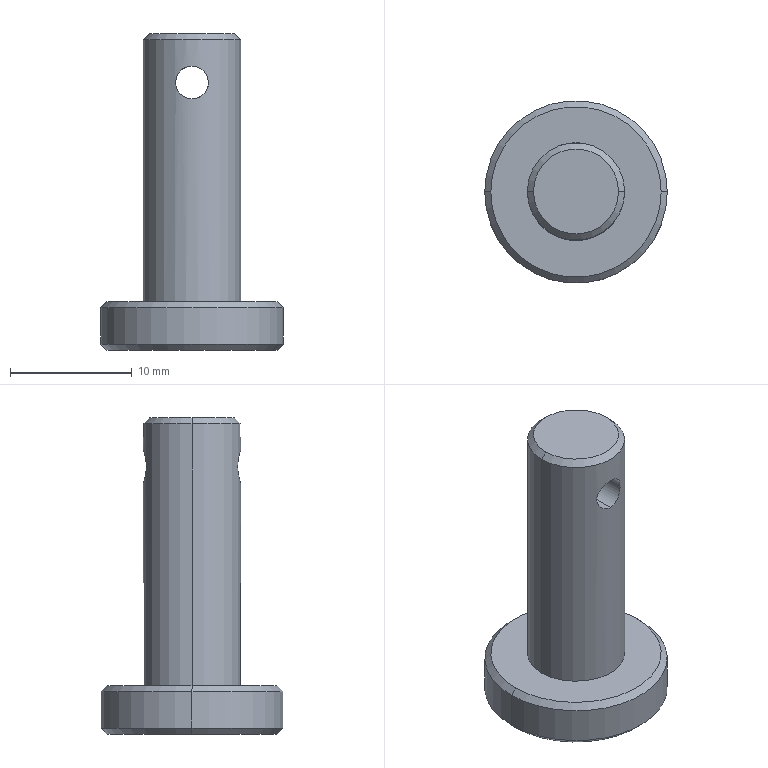Part | SolidWorks | features ICE 2, Chamfer 1, Extrusion 1 | 1 solid | 15 faces | box 15 x 15 x 26 mm | volume 1753 mm3 | cone 6 | cylinder 6 | plane 3 | commonest cylinder face diameters 2.7 x2 8 x2 15 x2
STEP:
#1=CARTESIAN_POINT('',(3.5,0.,22.));
#2=VERTEX_POINT('',#1);
#3=CARTESIAN_POINT('',(-3.5,0.,22.));
#4=VERTEX_POINT('',#3);
#5=CARTESIAN_POINT('',(0.,0.,22.));
#6=DIRECTION('',(0.,0.,1.));
#7=DIRECTION('',(1.,0.,0.));
#8=AXIS2_PLACEMENT_3D('',#5,#6,#7);
#9=CIRCLE('',#8,3.5);
#10=EDGE_CURVE('',#2,#4,#9,.T.);
#11=ORIENTED_EDGE('',*,*,#10,.F.);
#12=CARTESIAN_POINT('',(4.,0.,21.5));
#13=VERTEX_POINT('',#12);
#14=CARTESIAN_POINT('',(3.5,0.,22.));
#15=DIRECTION('',(0.7071,0.,-0.7071));
#16=VECTOR('',#15,1000.);
#17=LINE('',#14,#16);
#18=EDGE_CURVE('',#2,#13,#17,.T.);
#19=ORIENTED_EDGE('',*,*,#18,.T.);
#20=CARTESIAN_POINT('',(-4.,0.,21.5));
#21=VERTEX_POINT('',#20);
#22=CARTESIAN_POINT('',(0.,0.,21.5));
#23=DIRECTION('',(0.,0.,-1.));
#24=DIRECTION('',(1.,0.,0.));
#25=AXIS2_PLACEMENT_3D('',#22,#23,#24);
#26=CIRCLE('',#25,4.);
#27=EDGE_CURVE('',#21,#13,#26,.T.);
#28=ORIENTED_EDGE('',*,*,#27,.F.);
#29=CARTESIAN_POINT('',(-3.5,0.,22.));
#30=DIRECTION('',(-0.7071,0.,-0.7071));
#31=VECTOR('',#30,1000.);
#32=LINE('',#29,#31);
#33=EDGE_CURVE('',#4,#21,#32,.T.);
#34=ORIENTED_EDGE('',*,*,#33,.F.);
#35=EDGE_LOOP('',(#11,#19,#28,#34));
#36=FACE_OUTER_BOUND('',#35,.T.);
#37=CARTESIAN_POINT('',(0.,0.,22.));
#38=DIRECTION('',(0.,0.,-1.));
#39=DIRECTION('',(-1.,0.,0.));
#40=AXIS2_PLACEMENT_3D('',#37,#38,#39);
#41=CONICAL_SURFACE('',#40,3.5,0.7854);
#42=ADVANCED_FACE('',(#36),#41,.T.);
#43=CARTESIAN_POINT('',(7.,0.,0.));
#44=VERTEX_POINT('',#43);
#45=CARTESIAN_POINT('',(-7.,0.,0.));
#46=VERTEX_POINT('',#45);
#47=CARTESIAN_POINT('',(0.,0.,0.));
#48=DIRECTION('',(0.,0.,1.));
#49=DIRECTION('',(-1.,0.,0.));
#50=AXIS2_PLACEMENT_3D('',#47,#48,#49);
#51=CIRCLE('',#50,7.);
#52=EDGE_CURVE('',#44,#46,#51,.T.);
#53=ORIENTED_EDGE('',*,*,#52,.F.);
#54=CARTESIAN_POINT('',(7.5,0.,-0.5));
#55=VERTEX_POINT('',#54);
#56=CARTESIAN_POINT('',(7.5,0.,-0.5));
#57=DIRECTION('',(0.7071,0.,-0.7071));
#58=VECTOR('',#57,1000.);
#59=LINE('',#56,#58);
#60=EDGE_CURVE('',#44,#55,#59,.T.);
#61=ORIENTED_EDGE('',*,*,#60,.T.);
#62=CARTESIAN_POINT('',(-7.5,0.,-0.5));
#63=VERTEX_POINT('',#62);
#64=CARTESIAN_POINT('',(0.,0.,-0.5));
#65=DIRECTION('',(0.,0.,-1.));
#66=DIRECTION('',(-1.,0.,0.));
#67=AXIS2_PLACEMENT_3D('',#64,#65,#66);
#68=CIRCLE('',#67,7.5);
#69=EDGE_CURVE('',#63,#55,#68,.T.);
#70=ORIENTED_EDGE('',*,*,#69,.F.);
#71=CARTESIAN_POINT('',(-7.5,0.,-0.5));
#72=DIRECTION('',(-0.7071,0.,-0.7071));
#73=VECTOR('',#72,1000.);
#74=LINE('',#71,#73);
#75=EDGE_CURVE('',#46,#63,#74,.T.);
#76=ORIENTED_EDGE('',*,*,#75,.F.);
#77=EDGE_LOOP('',(#53,#61,#70,#76));
#78=FACE_OUTER_BOUND('',#77,.T.);
#79=CARTESIAN_POINT('',(0.,0.,-0.5));
#80=DIRECTION('',(0.,0.,-1.));
#81=DIRECTION('',(-1.,0.,0.));
#82=AXIS2_PLACEMENT_3D('',#79,#80,#81);
#83=CONICAL_SURFACE('',#82,7.5,0.7854);
#84=ADVANCED_FACE('',(#78),#83,.T.);
#85=CARTESIAN_POINT('',(-7.,0.,-4.));
#86=VERTEX_POINT('',#85);
#87=CARTESIAN_POINT('',(7.,0.,-4.));
#88=VERTEX_POINT('',#87);
#89=CARTESIAN_POINT('',(0.,0.,-4.));
#90=DIRECTION('',(0.,0.,-1.));
#91=DIRECTION('',(-1.,0.,0.));
#92=AXIS2_PLACEMENT_3D('',#89,#90,#91);
#93=CIRCLE('',#92,7.);
#94=EDGE_CURVE('',#86,#88,#93,.T.);
#95=ORIENTED_EDGE('',*,*,#94,.F.);
#96=CARTESIAN_POINT('',(-7.5,0.,-3.5));
#97=VERTEX_POINT('',#96);
#98=CARTESIAN_POINT('',(-7.,0.,-4.));
#99=DIRECTION('',(-0.7071,0.,0.7071));
#100=VECTOR('',#99,1000.);
#101=LINE('',#98,#100);
#102=EDGE_CURVE('',#86,#97,#101,.T.);
#103=ORIENTED_EDGE('',*,*,#102,.T.);
#104=CARTESIAN_POINT('',(7.5,0.,-3.5));
#105=VERTEX_POINT('',#104);
#106=CARTESIAN_POINT('',(0.,0.,-3.5));
#107=DIRECTION('',(0.,0.,1.));
#108=DIRECTION('',(-1.,0.,0.));
#109=AXIS2_PLACEMENT_3D('',#106,#107,#108);
#110=CIRCLE('',#109,7.5);
#111=EDGE_CURVE('',#105,#97,#110,.T.);
#112=ORIENTED_EDGE('',*,*,#111,.F.);
#113=CARTESIAN_POINT('',(7.,0.,-4.));
#114=DIRECTION('',(0.7071,0.,0.7071));
#115=VECTOR('',#114,1000.);
#116=LINE('',#113,#115);
#117=EDGE_CURVE('',#88,#105,#116,.T.);
#118=ORIENTED_EDGE('',*,*,#117,.F.);
#119=EDGE_LOOP('',(#95,#103,#112,#118));
#120=FACE_OUTER_BOUND('',#119,.T.);
#121=CARTESIAN_POINT('',(0.,0.,-4.));
#122=DIRECTION('',(0.,0.,1.));
#123=DIRECTION('',(1.,0.,0.));
#124=AXIS2_PLACEMENT_3D('',#121,#122,#123);
#125=CONICAL_SURFACE('',#124,7.,0.7854);
#126=ADVANCED_FACE('',(#120),#125,.T.);
#127=CARTESIAN_POINT('',(0.,-4.,16.65));
#128=VERTEX_POINT('',#127);
#129=CARTESIAN_POINT('',(0.,-4.,19.35));
#130=VERTEX_POINT('',#129);
#131=CARTESIAN_POINT('',(0.,-4.,16.65));
#132=CARTESIAN_POINT('',(-0.1771,-4.,16.65));
#133=CARTESIAN_POINT('',(-0.3558,-3.988,16.686));
#134=CARTESIAN_POINT('',(-0.6002,-3.956,16.788));
#135=CARTESIAN_POINT('',(-0.6792,-3.943,16.83));
#136=CARTESIAN_POINT('',(-0.8249,-3.915,16.928));
#137=CARTESIAN_POINT('',(-0.8925,-3.9,16.983));
#138=CARTESIAN_POINT('',(-1.079,-3.854,17.17));
#139=CARTESIAN_POINT('',(-1.178,-3.823,17.318));
#140=CARTESIAN_POINT('',(-1.281,-3.79,17.564));
#141=CARTESIAN_POINT('',(-1.306,-3.781,17.648));
#142=CARTESIAN_POINT('',(-1.341,-3.769,17.821));
#143=CARTESIAN_POINT('',(-1.35,-3.765,17.911));
#144=CARTESIAN_POINT('',(-1.35,-3.765,18.178));
#145=CARTESIAN_POINT('',(-1.314,-3.779,18.356));
#146=CARTESIAN_POINT('',(-1.179,-3.823,18.681));
#147=CARTESIAN_POINT('',(-1.078,-3.854,18.831));
#148=CARTESIAN_POINT('',(-0.8929,-3.9,19.016));
#149=CARTESIAN_POINT('',(-0.8239,-3.915,19.073));
#150=CARTESIAN_POINT('',(-0.6781,-3.943,19.171));
#151=CARTESIAN_POINT('',(-0.6009,-3.955,19.212));
#152=CARTESIAN_POINT('',(-0.4376,-3.977,19.28));
#153=CARTESIAN_POINT('',(-0.3516,-3.985,19.306));
#154=CARTESIAN_POINT('',(-0.1782,-3.997,19.341));
#155=CARTESIAN_POINT('',(-0.08989,-4.,19.35));
#156=CARTESIAN_POINT('',(0.,-4.,19.35));
#157=B_SPLINE_CURVE_WITH_KNOTS('',3,(#131,#132,#133,#134,#135,#136,#137,#138,#139,#140,#141,#142,#143,#144,#145,#146,#147,#148,#149,#150,#151,#152,#153,#154,#155,#156),.UNSPECIFIED.,.F.,.F.,(4,2,2,2,2,2,2,2,2,2,2,2,4),(0.004252,0.004784,0.005049,0.005315,0.005846,0.006112,0.006378,0.006909,0.007441,0.007706,0.007972,0.008238,0.008503),.UNSPECIFIED.);
#158=EDGE_CURVE('',#128,#130,#157,.T.);
#159=ORIENTED_EDGE('',*,*,#158,.F.);
#160=CARTESIAN_POINT('',(0.,4.,16.65));
#161=VERTEX_POINT('',#160);
#162=CARTESIAN_POINT('',(0.,-7.5,16.65));
#163=DIRECTION('',(0.,1.,0.));
#164=VECTOR('',#163,1000.);
#165=LINE('',#162,#164);
#166=EDGE_CURVE('',#128,#161,#165,.T.);
#167=ORIENTED_EDGE('',*,*,#166,.T.);
#168=CARTESIAN_POINT('',(0.,4.,19.35));
#169=VERTEX_POINT('',#168);
#170=CARTESIAN_POINT('',(0.,4.,19.35));
#171=CARTESIAN_POINT('',(-0.08991,4.,19.35));
#172=CARTESIAN_POINT('',(-0.1782,3.997,19.341));
#173=CARTESIAN_POINT('',(-0.3517,3.985,19.306));
#174=CARTESIAN_POINT('',(-0.4378,3.977,19.28));
#175=CARTESIAN_POINT('',(-0.6826,3.945,19.178));
#176=CARTESIAN_POINT('',(-0.8315,3.915,19.078));
#177=CARTESIAN_POINT('',(-1.079,3.854,18.831));
#178=CARTESIAN_POINT('',(-1.179,3.823,18.681));
#179=CARTESIAN_POINT('',(-1.314,3.779,18.357));
#180=CARTESIAN_POINT('',(-1.35,3.765,18.178));
#181=CARTESIAN_POINT('',(-1.35,3.765,17.912));
#182=CARTESIAN_POINT('',(-1.341,3.769,17.822));
#183=CARTESIAN_POINT('',(-1.306,3.781,17.648));
#184=CARTESIAN_POINT('',(-1.281,3.79,17.563));
#185=CARTESIAN_POINT('',(-1.178,3.823,17.317));
#186=CARTESIAN_POINT('',(-1.078,3.854,17.169));
#187=CARTESIAN_POINT('',(-0.8921,3.9,16.983));
#188=CARTESIAN_POINT('',(-0.8246,3.915,16.928));
#189=CARTESIAN_POINT('',(-0.6788,3.943,16.83));
#190=CARTESIAN_POINT('',(-0.5998,3.956,16.787));
#191=CARTESIAN_POINT('',(-0.3559,3.988,16.686));
#192=CARTESIAN_POINT('',(-0.1771,4.,16.65));
#193=CARTESIAN_POINT('',(0.,4.,16.65));
#194=B_SPLINE_CURVE_WITH_KNOTS('',3,(#170,#171,#172,#173,#174,#175,#176,#177,#178,#179,#180,#181,#182,#183,#184,#185,#186,#187,#188,#189,#190,#191,#192,#193),.UNSPECIFIED.,.F.,.F.,(4,2,2,2,2,2,2,2,2,2,2,4),(0.,0.0002658,0.0005315,0.001063,0.001595,0.002126,0.002392,0.002658,0.003189,0.003455,0.003721,0.004252),.UNSPECIFIED.);
#195=EDGE_CURVE('',#169,#161,#194,.T.);
#196=ORIENTED_EDGE('',*,*,#195,.F.);
#197=CARTESIAN_POINT('',(0.,-7.5,19.35));
#198=DIRECTION('',(0.,1.,0.));
#199=VECTOR('',#198,1000.);
#200=LINE('',#197,#199);
#201=EDGE_CURVE('',#130,#169,#200,.T.);
#202=ORIENTED_EDGE('',*,*,#201,.F.);
#203=EDGE_LOOP('',(#159,#167,#196,#202));
#204=FACE_OUTER_BOUND('',#203,.T.);
#205=CARTESIAN_POINT('',(0.,-7.5,18.));
#206=DIRECTION('',(0.,1.,0.));
#207=DIRECTION('',(0.,0.,1.));
#208=AXIS2_PLACEMENT_3D('',#205,#206,#207);
#209=CYLINDRICAL_SURFACE('',#208,1.35);
#210=ADVANCED_FACE('',(#204),#209,.F.);
#211=ORIENTED_EDGE('',*,*,#111,.T.);
#212=CARTESIAN_POINT('',(-7.5,0.,-4.));
#213=DIRECTION('',(0.,0.,1.));
#214=VECTOR('',#213,1000.);
#215=LINE('',#212,#214);
#216=EDGE_CURVE('',#97,#63,#215,.T.);
#217=ORIENTED_EDGE('',*,*,#216,.T.);
#218=ORIENTED_EDGE('',*,*,#69,.T.);
#219=CARTESIAN_POINT('',(7.5,0.,-4.));
#220=DIRECTION('',(0.,0.,1.));
#221=VECTOR('',#220,1000.);
#222=LINE('',#219,#221);
#223=EDGE_CURVE('',#105,#55,#222,.T.);
#224=ORIENTED_EDGE('',*,*,#223,.F.);
#225=EDGE_LOOP('',(#211,#217,#218,#224));
#226=FACE_OUTER_BOUND('',#225,.T.);
#227=CARTESIAN_POINT('',(0.,0.,-4.));
#228=DIRECTION('',(0.,0.,1.));
#229=DIRECTION('',(1.,0.,0.));
#230=AXIS2_PLACEMENT_3D('',#227,#228,#229);
#231=CYLINDRICAL_SURFACE('',#230,7.5);
#232=ADVANCED_FACE('',(#226),#231,.T.);
#233=ORIENTED_EDGE('',*,*,#195,.T.);
#234=CARTESIAN_POINT('',(0.,4.,16.65));
#235=CARTESIAN_POINT('',(0.1771,4.,16.65));
#236=CARTESIAN_POINT('',(0.3558,3.988,16.686));
#237=CARTESIAN_POINT('',(0.6002,3.956,16.788));
#238=CARTESIAN_POINT('',(0.6792,3.943,16.83));
#239=CARTESIAN_POINT('',(0.8249,3.915,16.928));
#240=CARTESIAN_POINT('',(0.8925,3.9,16.983));
#241=CARTESIAN_POINT('',(1.079,3.854,17.17));
#242=CARTESIAN_POINT('',(1.178,3.823,17.318));
#243=CARTESIAN_POINT('',(1.281,3.79,17.564));
#244=CARTESIAN_POINT('',(1.306,3.781,17.648));
#245=CARTESIAN_POINT('',(1.341,3.769,17.821));
#246=CARTESIAN_POINT('',(1.35,3.765,17.911));
#247=CARTESIAN_POINT('',(1.35,3.765,18.178));
#248=CARTESIAN_POINT('',(1.314,3.779,18.356));
#249=CARTESIAN_POINT('',(1.179,3.823,18.681));
#250=CARTESIAN_POINT('',(1.078,3.854,18.831));
#251=CARTESIAN_POINT('',(0.8929,3.9,19.016));
#252=CARTESIAN_POINT('',(0.8239,3.915,19.073));
#253=CARTESIAN_POINT('',(0.6781,3.943,19.171));
#254=CARTESIAN_POINT('',(0.6009,3.955,19.212));
#255=CARTESIAN_POINT('',(0.4376,3.977,19.28));
#256=CARTESIAN_POINT('',(0.3516,3.985,19.306));
#257=CARTESIAN_POINT('',(0.1782,3.997,19.341));
#258=CARTESIAN_POINT('',(0.08989,4.,19.35));
#259=CARTESIAN_POINT('',(0.,4.,19.35));
#260=B_SPLINE_CURVE_WITH_KNOTS('',3,(#234,#235,#236,#237,#238,#239,#240,#241,#242,#243,#244,#245,#246,#247,#248,#249,#250,#251,#252,#253,#254,#255,#256,#257,#258,#259),.UNSPECIFIED.,.F.,.F.,(4,2,2,2,2,2,2,2,2,2,2,2,4),(0.004252,0.004784,0.005049,0.005315,0.005846,0.006112,0.006378,0.006909,0.007441,0.007706,0.007972,0.008238,0.008503),.UNSPECIFIED.);
#261=EDGE_CURVE('',#161,#169,#260,.T.);
#262=ORIENTED_EDGE('',*,*,#261,.T.);
#263=EDGE_LOOP('',(#233,#262));
#264=FACE_BOUND('',#263,.T.);
#265=ORIENTED_EDGE('',*,*,#27,.T.);
#266=CARTESIAN_POINT('',(4.,0.,0.));
#267=VERTEX_POINT('',#266);
#268=CARTESIAN_POINT('',(4.,0.,22.));
#269=DIRECTION('',(0.,0.,-1.));
#270=VECTOR('',#269,1000.);
#271=LINE('',#268,#270);
#272=EDGE_CURVE('',#13,#267,#271,.T.);
#273=ORIENTED_EDGE('',*,*,#272,.T.);
#274=CARTESIAN_POINT('',(-4.,0.,0.));
#275=VERTEX_POINT('',#274);
#276=CARTESIAN_POINT('',(0.,0.,0.));
#277=DIRECTION('',(0.,0.,1.));
#278=DIRECTION('',(1.,0.,0.));
#279=AXIS2_PLACEMENT_3D('',#276,#277,#278);
#280=CIRCLE('',#279,4.);
#281=EDGE_CURVE('',#267,#275,#280,.T.);
#282=ORIENTED_EDGE('',*,*,#281,.T.);
#283=CARTESIAN_POINT('',(-4.,0.,22.));
#284=DIRECTION('',(0.,0.,-1.));
#285=VECTOR('',#284,1000.);
#286=LINE('',#283,#285);
#287=EDGE_CURVE('',#21,#275,#286,.T.);
#288=ORIENTED_EDGE('',*,*,#287,.F.);
#289=EDGE_LOOP('',(#265,#273,#282,#288));
#290=FACE_OUTER_BOUND('',#289,.T.);
#291=CARTESIAN_POINT('',(0.,0.,22.));
#292=DIRECTION('',(0.,0.,-1.));
#293=DIRECTION('',(-1.,0.,0.));
#294=AXIS2_PLACEMENT_3D('',#291,#292,#293);
#295=CYLINDRICAL_SURFACE('',#294,4.);
#296=ADVANCED_FACE('',(#264,#290),#295,.T.);
#297=ORIENTED_EDGE('',*,*,#272,.F.);
#298=CARTESIAN_POINT('',(0.,0.,21.5));
#299=DIRECTION('',(0.,0.,-1.));
#300=DIRECTION('',(1.,0.,0.));
#301=AXIS2_PLACEMENT_3D('',#298,#299,#300);
#302=CIRCLE('',#301,4.);
#303=EDGE_CURVE('',#13,#21,#302,.T.);
#304=ORIENTED_EDGE('',*,*,#303,.T.);
#305=ORIENTED_EDGE('',*,*,#287,.T.);
#306=CARTESIAN_POINT('',(0.,0.,0.));
#307=DIRECTION('',(0.,0.,1.));
#308=DIRECTION('',(1.,0.,0.));
#309=AXIS2_PLACEMENT_3D('',#306,#307,#308);
#310=CIRCLE('',#309,4.);
#311=EDGE_CURVE('',#275,#267,#310,.T.);
#312=ORIENTED_EDGE('',*,*,#311,.T.);
#313=EDGE_LOOP('',(#297,#304,#305,#312));
#314=FACE_OUTER_BOUND('',#313,.T.);
#315=CARTESIAN_POINT('',(0.,-4.,19.35));
#316=CARTESIAN_POINT('',(0.08991,-4.,19.35));
#317=CARTESIAN_POINT('',(0.1782,-3.997,19.341));
#318=CARTESIAN_POINT('',(0.3517,-3.985,19.306));
#319=CARTESIAN_POINT('',(0.4378,-3.977,19.28));
#320=CARTESIAN_POINT('',(0.6826,-3.945,19.178));
#321=CARTESIAN_POINT('',(0.8315,-3.915,19.078));
#322=CARTESIAN_POINT('',(1.079,-3.854,18.831));
#323=CARTESIAN_POINT('',(1.179,-3.823,18.681));
#324=CARTESIAN_POINT('',(1.314,-3.779,18.357));
#325=CARTESIAN_POINT('',(1.35,-3.765,18.178));
#326=CARTESIAN_POINT('',(1.35,-3.765,17.912));
#327=CARTESIAN_POINT('',(1.341,-3.769,17.822));
#328=CARTESIAN_POINT('',(1.306,-3.781,17.648));
#329=CARTESIAN_POINT('',(1.281,-3.79,17.563));
#330=CARTESIAN_POINT('',(1.178,-3.823,17.317));
#331=CARTESIAN_POINT('',(1.078,-3.854,17.169));
#332=CARTESIAN_POINT('',(0.8921,-3.9,16.983));
#333=CARTESIAN_POINT('',(0.8246,-3.915,16.928));
#334=CARTESIAN_POINT('',(0.6788,-3.943,16.83));
#335=CARTESIAN_POINT('',(0.5998,-3.956,16.787));
#336=CARTESIAN_POINT('',(0.3559,-3.988,16.686));
#337=CARTESIAN_POINT('',(0.1771,-4.,16.65));
#338=CARTESIAN_POINT('',(0.,-4.,16.65));
#339=B_SPLINE_CURVE_WITH_KNOTS('',3,(#315,#316,#317,#318,#319,#320,#321,#322,#323,#324,#325,#326,#327,#328,#329,#330,#331,#332,#333,#334,#335,#336,#337,#338),.UNSPECIFIED.,.F.,.F.,(4,2,2,2,2,2,2,2,2,2,2,4),(0.,0.0002658,0.0005315,0.001063,0.001595,0.002126,0.002392,0.002658,0.003189,0.003455,0.003721,0.004252),.UNSPECIFIED.);
#340=EDGE_CURVE('',#130,#128,#339,.T.);
#341=ORIENTED_EDGE('',*,*,#340,.T.);
#342=ORIENTED_EDGE('',*,*,#158,.T.);
#343=EDGE_LOOP('',(#341,#342));
#344=FACE_BOUND('',#343,.T.);
#345=CARTESIAN_POINT('',(0.,0.,22.));
#346=DIRECTION('',(0.,0.,-1.));
#347=DIRECTION('',(-1.,0.,0.));
#348=AXIS2_PLACEMENT_3D('',#345,#346,#347);
#349=CYLINDRICAL_SURFACE('',#348,4.);
#350=ADVANCED_FACE('',(#314,#344),#349,.T.);
#351=CARTESIAN_POINT('',(0.,0.,22.));
#352=DIRECTION('',(0.,0.,1.));
#353=DIRECTION('',(1.,0.,0.));
#354=AXIS2_PLACEMENT_3D('',#351,#352,#353);
#355=CIRCLE('',#354,3.5);
#356=EDGE_CURVE('',#4,#2,#355,.T.);
#357=ORIENTED_EDGE('',*,*,#356,.T.);
#358=ORIENTED_EDGE('',*,*,#10,.T.);
#359=EDGE_LOOP('',(#357,#358));
#360=FACE_OUTER_BOUND('',#359,.T.);
#361=CARTESIAN_POINT('',(0.,0.,22.));
#362=DIRECTION('',(0.,0.,1.));
#363=DIRECTION('',(1.,0.,0.));
#364=AXIS2_PLACEMENT_3D('',#361,#362,#363);
#365=PLANE('',#364);
#366=ADVANCED_FACE('',(#360),#365,.T.);
#367=ORIENTED_EDGE('',*,*,#216,.F.);
#368=CARTESIAN_POINT('',(0.,0.,-3.5));
#369=DIRECTION('',(0.,0.,1.));
#370=DIRECTION('',(-1.,0.,0.));
#371=AXIS2_PLACEMENT_3D('',#368,#369,#370);
#372=CIRCLE('',#371,7.5);
#373=EDGE_CURVE('',#97,#105,#372,.T.);
#374=ORIENTED_EDGE('',*,*,#373,.T.);
#375=ORIENTED_EDGE('',*,*,#223,.T.);
#376=CARTESIAN_POINT('',(0.,0.,-0.5));
#377=DIRECTION('',(0.,0.,-1.));
#378=DIRECTION('',(-1.,0.,0.));
#379=AXIS2_PLACEMENT_3D('',#376,#377,#378);
#380=CIRCLE('',#379,7.5);
#381=EDGE_CURVE('',#55,#63,#380,.T.);
#382=ORIENTED_EDGE('',*,*,#381,.T.);
#383=EDGE_LOOP('',(#367,#374,#375,#382));
#384=FACE_OUTER_BOUND('',#383,.T.);
#385=CARTESIAN_POINT('',(0.,0.,-4.));
#386=DIRECTION('',(0.,0.,1.));
#387=DIRECTION('',(1.,0.,0.));
#388=AXIS2_PLACEMENT_3D('',#385,#386,#387);
#389=CYLINDRICAL_SURFACE('',#388,7.5);
#390=ADVANCED_FACE('',(#384),#389,.T.);
#391=CARTESIAN_POINT('',(0.,0.,-4.));
#392=DIRECTION('',(0.,0.,-1.));
#393=DIRECTION('',(-1.,0.,0.));
#394=AXIS2_PLACEMENT_3D('',#391,#392,#393);
#395=CIRCLE('',#394,7.);
#396=EDGE_CURVE('',#88,#86,#395,.T.);
#397=ORIENTED_EDGE('',*,*,#396,.T.);
#398=ORIENTED_EDGE('',*,*,#94,.T.);
#399=EDGE_LOOP('',(#397,#398));
#400=FACE_OUTER_BOUND('',#399,.T.);
#401=CARTESIAN_POINT('',(0.,0.,-4.));
#402=DIRECTION('',(0.,0.,-1.));
#403=DIRECTION('',(-1.,0.,0.));
#404=AXIS2_PLACEMENT_3D('',#401,#402,#403);
#405=PLANE('',#404);
#406=ADVANCED_FACE('',(#400),#405,.T.);
#407=CARTESIAN_POINT('',(0.,0.,0.));
#408=DIRECTION('',(0.,0.,1.));
#409=DIRECTION('',(-1.,0.,0.));
#410=AXIS2_PLACEMENT_3D('',#407,#408,#409);
#411=CIRCLE('',#410,7.);
#412=EDGE_CURVE('',#46,#44,#411,.T.);
#413=ORIENTED_EDGE('',*,*,#412,.T.);
#414=ORIENTED_EDGE('',*,*,#52,.T.);
#415=EDGE_LOOP('',(#413,#414));
#416=FACE_OUTER_BOUND('',#415,.T.);
#417=ORIENTED_EDGE('',*,*,#311,.F.);
#418=ORIENTED_EDGE('',*,*,#281,.F.);
#419=EDGE_LOOP('',(#417,#418));
#420=FACE_BOUND('',#419,.T.);
#421=CARTESIAN_POINT('',(0.,0.,0.));
#422=DIRECTION('',(0.,0.,-1.));
#423=DIRECTION('',(-1.,0.,0.));
#424=AXIS2_PLACEMENT_3D('',#421,#422,#423);
#425=PLANE('',#424);
#426=ADVANCED_FACE('',(#416,#420),#425,.F.);
#427=ORIENTED_EDGE('',*,*,#166,.F.);
#428=ORIENTED_EDGE('',*,*,#340,.F.);
#429=ORIENTED_EDGE('',*,*,#201,.T.);
#430=ORIENTED_EDGE('',*,*,#261,.F.);
#431=EDGE_LOOP('',(#427,#428,#429,#430));
#432=FACE_OUTER_BOUND('',#431,.T.);
#433=CARTESIAN_POINT('',(0.,-7.5,18.));
#434=DIRECTION('',(0.,1.,0.));
#435=DIRECTION('',(0.,0.,1.));
#436=AXIS2_PLACEMENT_3D('',#433,#434,#435);
#437=CYLINDRICAL_SURFACE('',#436,1.35);
#438=ADVANCED_FACE('',(#432),#437,.F.);
#439=ORIENTED_EDGE('',*,*,#102,.F.);
#440=ORIENTED_EDGE('',*,*,#396,.F.);
#441=ORIENTED_EDGE('',*,*,#117,.T.);
#442=ORIENTED_EDGE('',*,*,#373,.F.);
#443=EDGE_LOOP('',(#439,#440,#441,#442));
#444=FACE_OUTER_BOUND('',#443,.T.);
#445=CARTESIAN_POINT('',(0.,0.,-4.));
#446=DIRECTION('',(0.,0.,1.));
#447=DIRECTION('',(1.,0.,0.));
#448=AXIS2_PLACEMENT_3D('',#445,#446,#447);
#449=CONICAL_SURFACE('',#448,7.,0.7854);
#450=ADVANCED_FACE('',(#444),#449,.T.);
#451=ORIENTED_EDGE('',*,*,#60,.F.);
#452=ORIENTED_EDGE('',*,*,#412,.F.);
#453=ORIENTED_EDGE('',*,*,#75,.T.);
#454=ORIENTED_EDGE('',*,*,#381,.F.);
#455=EDGE_LOOP('',(#451,#452,#453,#454));
#456=FACE_OUTER_BOUND('',#455,.T.);
#457=CARTESIAN_POINT('',(0.,0.,-0.5));
#458=DIRECTION('',(0.,0.,-1.));
#459=DIRECTION('',(-1.,0.,0.));
#460=AXIS2_PLACEMENT_3D('',#457,#458,#459);
#461=CONICAL_SURFACE('',#460,7.5,0.7854);
#462=ADVANCED_FACE('',(#456),#461,.T.);
#463=ORIENTED_EDGE('',*,*,#18,.F.);
#464=ORIENTED_EDGE('',*,*,#356,.F.);
#465=ORIENTED_EDGE('',*,*,#33,.T.);
#466=ORIENTED_EDGE('',*,*,#303,.F.);
#467=EDGE_LOOP('',(#463,#464,#465,#466));
#468=FACE_OUTER_BOUND('',#467,.T.);
#469=CARTESIAN_POINT('',(0.,0.,22.));
#470=DIRECTION('',(0.,0.,-1.));
#471=DIRECTION('',(-1.,0.,0.));
#472=AXIS2_PLACEMENT_3D('',#469,#470,#471);
#473=CONICAL_SURFACE('',#472,3.5,0.7854);
#474=ADVANCED_FACE('',(#468),#473,.T.);
#475=CLOSED_SHELL('',(#42,#84,#126,#210,#232,#296,#350,#366,#390,#406,#426,#438,#450,#462,#474));
#476=MANIFOLD_SOLID_BREP('',#475);
#477=CARTESIAN_POINT('',(0.,0.,0.));
#478=DIRECTION('',(0.,0.,1.));
#479=DIRECTION('',(1.,0.,0.));
#480=AXIS2_PLACEMENT_3D('',#477,#478,#479);
#481=(LENGTH_UNIT()NAMED_UNIT(*)SI_UNIT(.MILLI.,.METRE.));
#482=UNCERTAINTY_MEASURE_WITH_UNIT(LENGTH_MEASURE(0.00001),#481,'','');
#483=(NAMED_UNIT(*)PLANE_ANGLE_UNIT()SI_UNIT($,.RADIAN.));
#484=(NAMED_UNIT(*)SI_UNIT($,.STERADIAN.)SOLID_ANGLE_UNIT());
#485=(GEOMETRIC_REPRESENTATION_CONTEXT(3)GLOBAL_UNCERTAINTY_ASSIGNED_CONTEXT((#482))GLOBAL_UNIT_ASSIGNED_CONTEXT((#481,#483,#484))REPRESENTATION_CONTEXT('',''));
#486=ADVANCED_BREP_SHAPE_REPRESENTATION('',(#476,#480),#485);